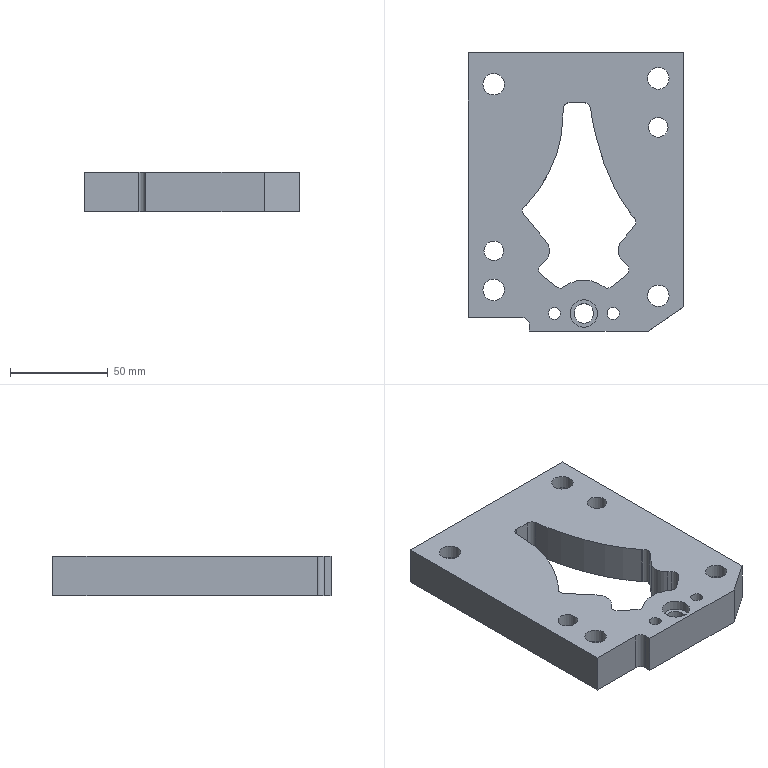Part | STEP file | 409_id3158_x_t | 1 solid | 56 faces | box 110 x 142 x 20 mm | volume 222515 mm3 | cylinder 30 | plane 23 | spline 3 | commonest cylinder face diameters 6 x6 11 x6 17 x4 7 x3 10 x3 4 x2